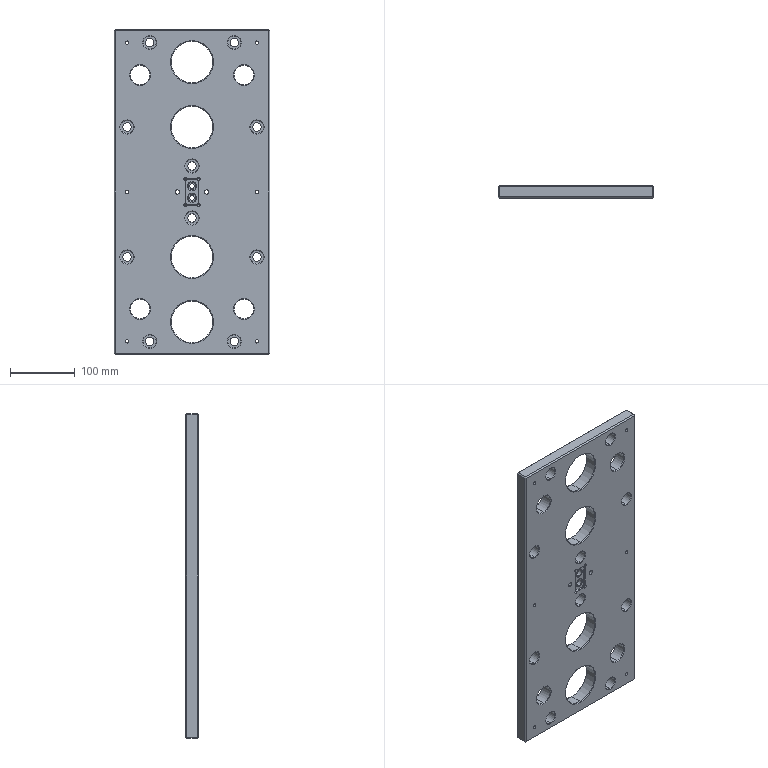Part | STEP file | PI - Torre - 1 cav | 1 solid | 221 faces | box 240 x 20 x 500 mm | volume 2015685 mm3 | cylinder 88 | cone 86 | plane 47 | commonest cylinder face diameters 5 x20 13 x20 20 x20 30 x8 64 x8 6.8 x4